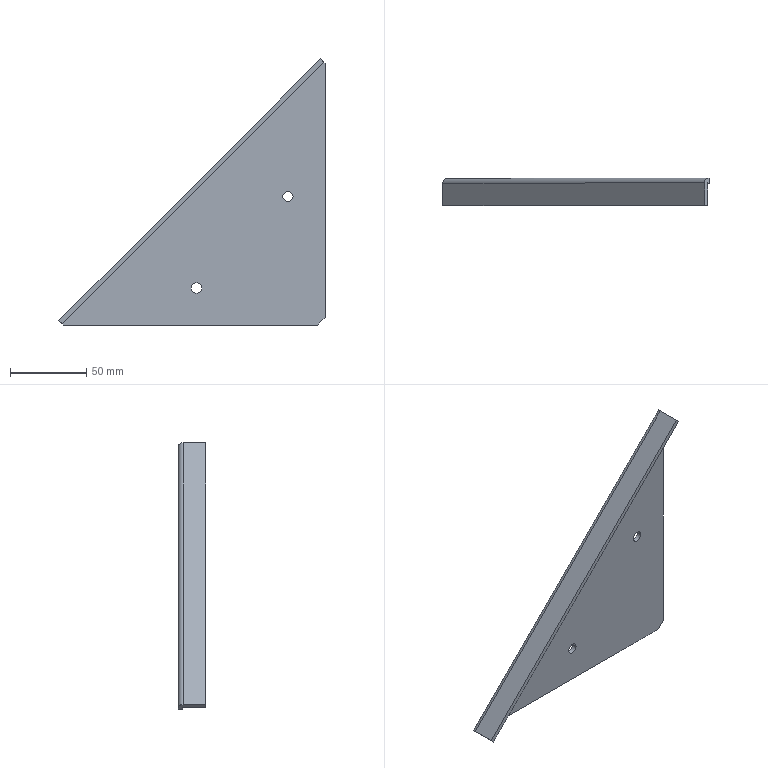Part | STEP file | HESS-408-70-15W-W-18-bottom frame triangular plate | 1 solid | 16 faces | box 175 x 18 x 175 mm | volume 57661 mm3 | plane 10 | cylinder 6 | commonest cylinder face diameters 6.8 x4 0.2 x1 6.2 x1
STEP:
#1=CARTESIAN_POINT('',(0.,0.,0.));
#2=DIRECTION('',(0.,0.,1.));
#3=DIRECTION('',(1.,0.,0.));
#4=AXIS2_PLACEMENT_3D('',#1,#2,#3);
#5=CARTESIAN_POINT('',(-27.826,-3.,84.53));
#6=VERTEX_POINT('',#5);
#7=CARTESIAN_POINT('',(-27.826,0.,84.53));
#8=VERTEX_POINT('',#7);
#9=CARTESIAN_POINT('',(-27.826,0.,84.53));
#10=DIRECTION('',(0.,1.,0.));
#11=VECTOR('',#10,1.);
#12=LINE('',#9,#11);
#13=CARTESIAN_POINT('',(-24.426,0.,84.53));
#14=DIRECTION('',(0.,1.,0.));
#15=DIRECTION('',(-1.,0.,0.));
#16=AXIS2_PLACEMENT_3D('',#13,#14,#15);
#17=CYLINDRICAL_SURFACE('',#16,3.4);
#18=CARTESIAN_POINT('',(6.283,0.));
#19=DIRECTION('',(0.,1.));
#20=VECTOR('',#19,1.);
#21=LINE('',#18,#20);
#22=(GEOMETRIC_REPRESENTATION_CONTEXT(2)PARAMETRIC_REPRESENTATION_CONTEXT()REPRESENTATION_CONTEXT('',''));
#23=DEFINITIONAL_REPRESENTATION('',(#21),#22);
#24=PCURVE('',#17,#23);
#25=CARTESIAN_POINT('',(-24.426,0.,84.53));
#26=DIRECTION('',(0.,1.,0.));
#27=DIRECTION('',(-1.,0.,0.));
#28=AXIS2_PLACEMENT_3D('',#25,#26,#27);
#29=CYLINDRICAL_SURFACE('',#28,3.4);
#30=CARTESIAN_POINT('',(0.,0.));
#31=DIRECTION('',(0.,1.));
#32=VECTOR('',#31,1.);
#33=LINE('',#30,#32);
#34=(GEOMETRIC_REPRESENTATION_CONTEXT(2)PARAMETRIC_REPRESENTATION_CONTEXT()REPRESENTATION_CONTEXT('',''));
#35=DEFINITIONAL_REPRESENTATION('',(#33),#34);
#36=PCURVE('',#29,#35);
#37=SURFACE_CURVE('',#12,(#24,#36),.PCURVE_S1.);
#38=EDGE_CURVE('',#6,#8,#37,.T.);
#39=ORIENTED_EDGE('',*,*,#38,.T.);
#40=CARTESIAN_POINT('',(-21.026,0.,84.53));
#41=VERTEX_POINT('',#40);
#42=CARTESIAN_POINT('',(-24.426,0.,84.53));
#43=DIRECTION('',(0.,-1.,0.));
#44=DIRECTION('',(-1.,0.,0.));
#45=AXIS2_PLACEMENT_3D('',#42,#43,#44);
#46=CIRCLE('',#45,3.4);
#47=CARTESIAN_POINT('',(6.283,0.));
#48=DIRECTION('',(-1.,0.));
#49=VECTOR('',#48,1.);
#50=LINE('',#47,#49);
#51=(GEOMETRIC_REPRESENTATION_CONTEXT(2)PARAMETRIC_REPRESENTATION_CONTEXT()REPRESENTATION_CONTEXT('',''));
#52=DEFINITIONAL_REPRESENTATION('',(#50),#51);
#53=PCURVE('',#17,#52);
#54=CARTESIAN_POINT('',(0.,0.,0.));
#55=DIRECTION('',(0.,1.,0.));
#56=DIRECTION('',(-1.,0.,0.));
#57=AXIS2_PLACEMENT_3D('',#54,#55,#56);
#58=PLANE('',#57);
#59=CARTESIAN_POINT('',(27.826,84.53));
#60=CARTESIAN_POINT('',(27.826,78.642));
#61=CARTESIAN_POINT('',(22.726,81.586));
#62=CARTESIAN_POINT('',(17.626,84.53));
#63=CARTESIAN_POINT('',(22.726,87.475));
#64=CARTESIAN_POINT('',(27.826,90.419));
#65=CARTESIAN_POINT('',(27.826,84.53));
#66=(BOUNDED_CURVE()B_SPLINE_CURVE(2,(#59,#60,#61,#62,#63,#64,#65),.UNSPECIFIED.,.T.,.F.)B_SPLINE_CURVE_WITH_KNOTS((1,2,2,2,2,1),(-2.094,0.,2.094,4.189,6.283,8.378),.UNSPECIFIED.)CURVE()GEOMETRIC_REPRESENTATION_ITEM()RATIONAL_B_SPLINE_CURVE((1.,0.5,1.,0.5,1.,0.5,1.))REPRESENTATION_ITEM(''));
#67=(GEOMETRIC_REPRESENTATION_CONTEXT(2)PARAMETRIC_REPRESENTATION_CONTEXT()REPRESENTATION_CONTEXT('',''));
#68=DEFINITIONAL_REPRESENTATION('',(#66),#67);
#69=PCURVE('',#58,#68);
#70=SURFACE_CURVE('',#46,(#53,#69),.PCURVE_S1.);
#71=EDGE_CURVE('',#8,#41,#70,.T.);
#72=ORIENTED_EDGE('',*,*,#71,.T.);
#73=CARTESIAN_POINT('',(-21.026,-3.,84.53));
#74=VERTEX_POINT('',#73);
#75=CARTESIAN_POINT('',(-21.026,0.,84.53));
#76=DIRECTION('',(0.,1.,0.));
#77=VECTOR('',#76,1.);
#78=LINE('',#75,#77);
#79=CARTESIAN_POINT('',(3.142,0.));
#80=DIRECTION('',(0.,1.));
#81=VECTOR('',#80,1.);
#82=LINE('',#79,#81);
#83=(GEOMETRIC_REPRESENTATION_CONTEXT(2)PARAMETRIC_REPRESENTATION_CONTEXT()REPRESENTATION_CONTEXT('',''));
#84=DEFINITIONAL_REPRESENTATION('',(#82),#83);
#85=PCURVE('',#17,#84);
#86=CARTESIAN_POINT('',(3.142,0.));
#87=DIRECTION('',(0.,1.));
#88=VECTOR('',#87,1.);
#89=LINE('',#86,#88);
#90=(GEOMETRIC_REPRESENTATION_CONTEXT(2)PARAMETRIC_REPRESENTATION_CONTEXT()REPRESENTATION_CONTEXT('',''));
#91=DEFINITIONAL_REPRESENTATION('',(#89),#90);
#92=PCURVE('',#29,#91);
#93=SURFACE_CURVE('',#78,(#85,#92),.PCURVE_S1.);
#94=EDGE_CURVE('',#74,#41,#93,.T.);
#95=ORIENTED_EDGE('',*,*,#94,.F.);
#96=CARTESIAN_POINT('',(-24.426,-3.,84.53));
#97=DIRECTION('',(0.,1.,0.));
#98=DIRECTION('',(-1.,0.,0.));
#99=AXIS2_PLACEMENT_3D('',#96,#97,#98);
#100=CIRCLE('',#99,3.4);
#101=CARTESIAN_POINT('',(0.,-3.));
#102=DIRECTION('',(1.,0.));
#103=VECTOR('',#102,1.);
#104=LINE('',#101,#103);
#105=(GEOMETRIC_REPRESENTATION_CONTEXT(2)PARAMETRIC_REPRESENTATION_CONTEXT()REPRESENTATION_CONTEXT('',''));
#106=DEFINITIONAL_REPRESENTATION('',(#104),#105);
#107=PCURVE('',#17,#106);
#108=CARTESIAN_POINT('',(0.,-3.,0.));
#109=DIRECTION('',(0.,1.,0.));
#110=DIRECTION('',(-1.,0.,0.));
#111=AXIS2_PLACEMENT_3D('',#108,#109,#110);
#112=PLANE('',#111);
#113=CARTESIAN_POINT('',(24.426,84.53));
#114=DIRECTION('',(1.,0.));
#115=AXIS2_PLACEMENT_2D('',#113,#114);
#116=CIRCLE('',#115,3.4);
#117=(GEOMETRIC_REPRESENTATION_CONTEXT(2)PARAMETRIC_REPRESENTATION_CONTEXT()REPRESENTATION_CONTEXT('',''));
#118=DEFINITIONAL_REPRESENTATION('',(#116),#117);
#119=PCURVE('',#112,#118);
#120=SURFACE_CURVE('',#100,(#107,#119),.PCURVE_S1.);
#121=EDGE_CURVE('',#74,#6,#120,.T.);
#122=ORIENTED_EDGE('',*,*,#121,.T.);
#123=EDGE_LOOP('',(#39,#72,#95,#122));
#124=FACE_BOUND('',#123,.F.);
#125=ADVANCED_FACE('',(#124),#17,.F.);
#126=CARTESIAN_POINT('',(-87.93,-3.,24.426));
#127=VERTEX_POINT('',#126);
#128=CARTESIAN_POINT('',(-87.93,0.,24.426));
#129=VERTEX_POINT('',#128);
#130=CARTESIAN_POINT('',(-87.93,0.,24.426));
#131=DIRECTION('',(0.,1.,0.));
#132=VECTOR('',#131,1.);
#133=LINE('',#130,#132);
#134=CARTESIAN_POINT('',(-84.53,0.,24.426));
#135=DIRECTION('',(0.,1.,0.));
#136=DIRECTION('',(-1.,0.,0.));
#137=AXIS2_PLACEMENT_3D('',#134,#135,#136);
#138=CYLINDRICAL_SURFACE('',#137,3.4);
#139=CARTESIAN_POINT('',(6.283,0.));
#140=DIRECTION('',(0.,1.));
#141=VECTOR('',#140,1.);
#142=LINE('',#139,#141);
#143=(GEOMETRIC_REPRESENTATION_CONTEXT(2)PARAMETRIC_REPRESENTATION_CONTEXT()REPRESENTATION_CONTEXT('',''));
#144=DEFINITIONAL_REPRESENTATION('',(#142),#143);
#145=PCURVE('',#138,#144);
#146=CARTESIAN_POINT('',(-84.53,0.,24.426));
#147=DIRECTION('',(0.,1.,0.));
#148=DIRECTION('',(-1.,0.,0.));
#149=AXIS2_PLACEMENT_3D('',#146,#147,#148);
#150=CYLINDRICAL_SURFACE('',#149,3.4);
#151=CARTESIAN_POINT('',(0.,0.));
#152=DIRECTION('',(0.,1.));
#153=VECTOR('',#152,1.);
#154=LINE('',#151,#153);
#155=(GEOMETRIC_REPRESENTATION_CONTEXT(2)PARAMETRIC_REPRESENTATION_CONTEXT()REPRESENTATION_CONTEXT('',''));
#156=DEFINITIONAL_REPRESENTATION('',(#154),#155);
#157=PCURVE('',#150,#156);
#158=SURFACE_CURVE('',#133,(#145,#157),.PCURVE_S1.);
#159=EDGE_CURVE('',#127,#129,#158,.T.);
#160=ORIENTED_EDGE('',*,*,#159,.T.);
#161=CARTESIAN_POINT('',(-81.13,0.,24.426));
#162=VERTEX_POINT('',#161);
#163=CARTESIAN_POINT('',(-84.53,0.,24.426));
#164=DIRECTION('',(0.,-1.,0.));
#165=DIRECTION('',(-1.,0.,0.));
#166=AXIS2_PLACEMENT_3D('',#163,#164,#165);
#167=CIRCLE('',#166,3.4);
#168=CARTESIAN_POINT('',(6.283,0.));
#169=DIRECTION('',(-1.,0.));
#170=VECTOR('',#169,1.);
#171=LINE('',#168,#170);
#172=(GEOMETRIC_REPRESENTATION_CONTEXT(2)PARAMETRIC_REPRESENTATION_CONTEXT()REPRESENTATION_CONTEXT('',''));
#173=DEFINITIONAL_REPRESENTATION('',(#171),#172);
#174=PCURVE('',#138,#173);
#175=CARTESIAN_POINT('',(87.93,24.426));
#176=CARTESIAN_POINT('',(87.93,18.537));
#177=CARTESIAN_POINT('',(82.83,21.482));
#178=CARTESIAN_POINT('',(77.73,24.426));
#179=CARTESIAN_POINT('',(82.83,27.371));
#180=CARTESIAN_POINT('',(87.93,30.315));
#181=CARTESIAN_POINT('',(87.93,24.426));
#182=(BOUNDED_CURVE()B_SPLINE_CURVE(2,(#175,#176,#177,#178,#179,#180,#181),.UNSPECIFIED.,.T.,.F.)B_SPLINE_CURVE_WITH_KNOTS((1,2,2,2,2,1),(-2.094,0.,2.094,4.189,6.283,8.378),.UNSPECIFIED.)CURVE()GEOMETRIC_REPRESENTATION_ITEM()RATIONAL_B_SPLINE_CURVE((1.,0.5,1.,0.5,1.,0.5,1.))REPRESENTATION_ITEM(''));
#183=(GEOMETRIC_REPRESENTATION_CONTEXT(2)PARAMETRIC_REPRESENTATION_CONTEXT()REPRESENTATION_CONTEXT('',''));
#184=DEFINITIONAL_REPRESENTATION('',(#182),#183);
#185=PCURVE('',#58,#184);
#186=SURFACE_CURVE('',#167,(#174,#185),.PCURVE_S1.);
#187=EDGE_CURVE('',#129,#162,#186,.T.);
#188=ORIENTED_EDGE('',*,*,#187,.T.);
#189=CARTESIAN_POINT('',(-81.13,-3.,24.426));
#190=VERTEX_POINT('',#189);
#191=CARTESIAN_POINT('',(-81.13,0.,24.426));
#192=DIRECTION('',(0.,1.,0.));
#193=VECTOR('',#192,1.);
#194=LINE('',#191,#193);
#195=CARTESIAN_POINT('',(3.142,0.));
#196=DIRECTION('',(0.,1.));
#197=VECTOR('',#196,1.);
#198=LINE('',#195,#197);
#199=(GEOMETRIC_REPRESENTATION_CONTEXT(2)PARAMETRIC_REPRESENTATION_CONTEXT()REPRESENTATION_CONTEXT('',''));
#200=DEFINITIONAL_REPRESENTATION('',(#198),#199);
#201=PCURVE('',#138,#200);
#202=CARTESIAN_POINT('',(3.142,0.));
#203=DIRECTION('',(0.,1.));
#204=VECTOR('',#203,1.);
#205=LINE('',#202,#204);
#206=(GEOMETRIC_REPRESENTATION_CONTEXT(2)PARAMETRIC_REPRESENTATION_CONTEXT()REPRESENTATION_CONTEXT('',''));
#207=DEFINITIONAL_REPRESENTATION('',(#205),#206);
#208=PCURVE('',#150,#207);
#209=SURFACE_CURVE('',#194,(#201,#208),.PCURVE_S1.);
#210=EDGE_CURVE('',#190,#162,#209,.T.);
#211=ORIENTED_EDGE('',*,*,#210,.F.);
#212=CARTESIAN_POINT('',(-84.53,-3.,24.426));
#213=DIRECTION('',(0.,1.,0.));
#214=DIRECTION('',(-1.,0.,0.));
#215=AXIS2_PLACEMENT_3D('',#212,#213,#214);
#216=CIRCLE('',#215,3.4);
#217=CARTESIAN_POINT('',(0.,-3.));
#218=DIRECTION('',(1.,0.));
#219=VECTOR('',#218,1.);
#220=LINE('',#217,#219);
#221=(GEOMETRIC_REPRESENTATION_CONTEXT(2)PARAMETRIC_REPRESENTATION_CONTEXT()REPRESENTATION_CONTEXT('',''));
#222=DEFINITIONAL_REPRESENTATION('',(#220),#221);
#223=PCURVE('',#138,#222);
#224=CARTESIAN_POINT('',(84.53,24.426));
#225=DIRECTION('',(1.,0.));
#226=AXIS2_PLACEMENT_2D('',#224,#225);
#227=CIRCLE('',#226,3.4);
#228=(GEOMETRIC_REPRESENTATION_CONTEXT(2)PARAMETRIC_REPRESENTATION_CONTEXT()REPRESENTATION_CONTEXT('',''));
#229=DEFINITIONAL_REPRESENTATION('',(#227),#228);
#230=PCURVE('',#112,#229);
#231=SURFACE_CURVE('',#216,(#223,#230),.PCURVE_S1.);
#232=EDGE_CURVE('',#190,#127,#231,.T.);
#233=ORIENTED_EDGE('',*,*,#232,.T.);
#234=EDGE_LOOP('',(#160,#188,#211,#233));
#235=FACE_BOUND('',#234,.F.);
#236=ADVANCED_FACE('',(#235),#138,.F.);
#237=CARTESIAN_POINT('',(-172.808,0.,0.808));
#238=VERTEX_POINT('',#237);
#239=CARTESIAN_POINT('',(-0.808,0.,172.808));
#240=VERTEX_POINT('',#239);
#241=CARTESIAN_POINT('',(-172.808,0.,0.808));
#242=DIRECTION('',(0.7071,0.,0.7071));
#243=VECTOR('',#242,1.);
#244=LINE('',#241,#243);
#245=CARTESIAN_POINT('',(172.808,0.808));
#246=DIRECTION('',(-0.7071,0.7071));
#247=VECTOR('',#246,1.);
#248=LINE('',#245,#247);
#249=(GEOMETRIC_REPRESENTATION_CONTEXT(2)PARAMETRIC_REPRESENTATION_CONTEXT()REPRESENTATION_CONTEXT('',''));
#250=DEFINITIONAL_REPRESENTATION('',(#248),#249);
#251=PCURVE('',#58,#250);
#252=CARTESIAN_POINT('',(-172.808,-3.1,0.808));
#253=DIRECTION('',(-0.7071,0.,-0.7071));
#254=DIRECTION('',(-0.7071,0.,0.7071));
#255=AXIS2_PLACEMENT_3D('',#252,#253,#254);
#256=CYLINDRICAL_SURFACE('',#255,3.1);
#257=CARTESIAN_POINT('',(1.571,0.));
#258=DIRECTION('',(0.,-1.));
#259=VECTOR('',#258,1.);
#260=LINE('',#257,#259);
#261=(GEOMETRIC_REPRESENTATION_CONTEXT(2)PARAMETRIC_REPRESENTATION_CONTEXT()REPRESENTATION_CONTEXT('',''));
#262=DEFINITIONAL_REPRESENTATION('',(#260),#261);
#263=PCURVE('',#256,#262);
#264=SURFACE_CURVE('',#244,(#251,#263),.PCURVE_S1.);
#265=EDGE_CURVE('',#238,#240,#264,.T.);
#266=ORIENTED_EDGE('',*,*,#265,.T.);
#267=CARTESIAN_POINT('',(0.,0.,172.));
#268=VERTEX_POINT('',#267);
#269=CARTESIAN_POINT('',(-0.808,0.,172.808));
#270=DIRECTION('',(-0.7071,0.,0.7071));
#271=VECTOR('',#270,1.);
#272=LINE('',#269,#271);
#273=CARTESIAN_POINT('',(0.808,172.808));
#274=DIRECTION('',(0.7071,0.7071));
#275=VECTOR('',#274,1.);
#276=LINE('',#273,#275);
#277=(GEOMETRIC_REPRESENTATION_CONTEXT(2)PARAMETRIC_REPRESENTATION_CONTEXT()REPRESENTATION_CONTEXT('',''));
#278=DEFINITIONAL_REPRESENTATION('',(#276),#277);
#279=PCURVE('',#58,#278);
#280=CARTESIAN_POINT('',(-0.808,-3.1,172.808));
#281=DIRECTION('',(0.7071,0.,0.7071));
#282=DIRECTION('',(0.7071,0.,-0.7071));
#283=AXIS2_PLACEMENT_3D('',#280,#281,#282);
#284=PLANE('',#283);
#285=CARTESIAN_POINT('',(0.,3.1));
#286=DIRECTION('',(-1.,0.));
#287=VECTOR('',#286,1.);
#288=LINE('',#285,#287);
#289=(GEOMETRIC_REPRESENTATION_CONTEXT(2)PARAMETRIC_REPRESENTATION_CONTEXT()REPRESENTATION_CONTEXT('',''));
#290=DEFINITIONAL_REPRESENTATION('',(#288),#289);
#291=PCURVE('',#284,#290);
#292=SURFACE_CURVE('',#272,(#279,#291),.PCURVE_S1.);
#293=EDGE_CURVE('',#268,#240,#292,.T.);
#294=ORIENTED_EDGE('',*,*,#293,.F.);
#295=CARTESIAN_POINT('',(0.,0.,5.));
#296=VERTEX_POINT('',#295);
#297=CARTESIAN_POINT('',(0.,0.,0.));
#298=DIRECTION('',(0.,0.,-1.));
#299=VECTOR('',#298,1.);
#300=LINE('',#297,#299);
#301=CARTESIAN_POINT('',(0.,0.));
#302=DIRECTION('',(0.,-1.));
#303=VECTOR('',#302,1.);
#304=LINE('',#301,#303);
#305=(GEOMETRIC_REPRESENTATION_CONTEXT(2)PARAMETRIC_REPRESENTATION_CONTEXT()REPRESENTATION_CONTEXT('',''));
#306=DEFINITIONAL_REPRESENTATION('',(#304),#305);
#307=PCURVE('',#58,#306);
#308=CARTESIAN_POINT('',(0.,-3.,175.));
#309=DIRECTION('',(1.,0.,0.));
#310=DIRECTION('',(0.,1.,0.));
#311=AXIS2_PLACEMENT_3D('',#308,#309,#310);
#312=PLANE('',#311);
#313=CARTESIAN_POINT('',(3.,-175.));
#314=DIRECTION('',(0.,-1.));
#315=VECTOR('',#314,1.);
#316=LINE('',#313,#315);
#317=(GEOMETRIC_REPRESENTATION_CONTEXT(2)PARAMETRIC_REPRESENTATION_CONTEXT()REPRESENTATION_CONTEXT('',''));
#318=DEFINITIONAL_REPRESENTATION('',(#316),#317);
#319=PCURVE('',#312,#318);
#320=SURFACE_CURVE('',#300,(#307,#319),.PCURVE_S1.);
#321=EDGE_CURVE('',#268,#296,#320,.T.);
#322=ORIENTED_EDGE('',*,*,#321,.T.);
#323=CARTESIAN_POINT('',(-5.,0.,0.));
#324=VERTEX_POINT('',#323);
#325=CARTESIAN_POINT('',(0.,0.,5.));
#326=DIRECTION('',(-0.7071,0.,-0.7071));
#327=VECTOR('',#326,1.);
#328=LINE('',#325,#327);
#329=CARTESIAN_POINT('',(0.,5.));
#330=DIRECTION('',(0.7071,-0.7071));
#331=VECTOR('',#330,1.);
#332=LINE('',#329,#331);
#333=(GEOMETRIC_REPRESENTATION_CONTEXT(2)PARAMETRIC_REPRESENTATION_CONTEXT()REPRESENTATION_CONTEXT('',''));
#334=DEFINITIONAL_REPRESENTATION('',(#332),#333);
#335=PCURVE('',#58,#334);
#336=CARTESIAN_POINT('',(0.,-3.,5.));
#337=DIRECTION('',(-0.7071,0.,0.7071));
#338=DIRECTION('',(0.7071,0.,0.7071));
#339=AXIS2_PLACEMENT_3D('',#336,#337,#338);
#340=PLANE('',#339);
#341=CARTESIAN_POINT('',(0.,3.));
#342=DIRECTION('',(-1.,0.));
#343=VECTOR('',#342,1.);
#344=LINE('',#341,#343);
#345=(GEOMETRIC_REPRESENTATION_CONTEXT(2)PARAMETRIC_REPRESENTATION_CONTEXT()REPRESENTATION_CONTEXT('',''));
#346=DEFINITIONAL_REPRESENTATION('',(#344),#345);
#347=PCURVE('',#340,#346);
#348=SURFACE_CURVE('',#328,(#335,#347),.PCURVE_S1.);
#349=EDGE_CURVE('',#296,#324,#348,.T.);
#350=ORIENTED_EDGE('',*,*,#349,.T.);
#351=CARTESIAN_POINT('',(-172.,0.,0.));
#352=VERTEX_POINT('',#351);
#353=CARTESIAN_POINT('',(0.,0.,0.));
#354=DIRECTION('',(-1.,0.,0.));
#355=VECTOR('',#354,1.);
#356=LINE('',#353,#355);
#357=CARTESIAN_POINT('',(0.,0.));
#358=DIRECTION('',(1.,0.));
#359=VECTOR('',#358,1.);
#360=LINE('',#357,#359);
#361=(GEOMETRIC_REPRESENTATION_CONTEXT(2)PARAMETRIC_REPRESENTATION_CONTEXT()REPRESENTATION_CONTEXT('',''));
#362=DEFINITIONAL_REPRESENTATION('',(#360),#361);
#363=PCURVE('',#58,#362);
#364=CARTESIAN_POINT('',(0.,-3.,0.));
#365=DIRECTION('',(0.,0.,-1.));
#366=DIRECTION('',(-1.,0.,0.));
#367=AXIS2_PLACEMENT_3D('',#364,#365,#366);
#368=PLANE('',#367);
#369=CARTESIAN_POINT('',(0.,3.));
#370=DIRECTION('',(1.,0.));
#371=VECTOR('',#370,1.);
#372=LINE('',#369,#371);
#373=(GEOMETRIC_REPRESENTATION_CONTEXT(2)PARAMETRIC_REPRESENTATION_CONTEXT()REPRESENTATION_CONTEXT('',''));
#374=DEFINITIONAL_REPRESENTATION('',(#372),#373);
#375=PCURVE('',#368,#374);
#376=SURFACE_CURVE('',#356,(#363,#375),.PCURVE_S1.);
#377=EDGE_CURVE('',#324,#352,#376,.T.);
#378=ORIENTED_EDGE('',*,*,#377,.T.);
#379=CARTESIAN_POINT('',(-172.596,0.,0.5958));
#380=DIRECTION('',(0.7071,0.,-0.7071));
#381=VECTOR('',#380,1.);
#382=LINE('',#379,#381);
#383=CARTESIAN_POINT('',(172.596,0.5958));
#384=DIRECTION('',(-0.7071,-0.7071));
#385=VECTOR('',#384,1.);
#386=LINE('',#383,#385);
#387=(GEOMETRIC_REPRESENTATION_CONTEXT(2)PARAMETRIC_REPRESENTATION_CONTEXT()REPRESENTATION_CONTEXT('',''));
#388=DEFINITIONAL_REPRESENTATION('',(#386),#387);
#389=PCURVE('',#58,#388);
#390=CARTESIAN_POINT('',(-172.808,-3.1,0.808));
#391=DIRECTION('',(0.7071,0.,0.7071));
#392=DIRECTION('',(0.7071,0.,-0.7071));
#393=AXIS2_PLACEMENT_3D('',#390,#391,#392);
#394=PLANE('',#393);
#395=CARTESIAN_POINT('',(0.3,3.1));
#396=DIRECTION('',(1.,0.));
#397=VECTOR('',#396,1.);
#398=LINE('',#395,#397);
#399=(GEOMETRIC_REPRESENTATION_CONTEXT(2)PARAMETRIC_REPRESENTATION_CONTEXT()REPRESENTATION_CONTEXT('',''));
#400=DEFINITIONAL_REPRESENTATION('',(#398),#399);
#401=PCURVE('',#394,#400);
#402=SURFACE_CURVE('',#382,(#389,#401),.PCURVE_S1.);
#403=EDGE_CURVE('',#238,#352,#402,.T.);
#404=ORIENTED_EDGE('',*,*,#403,.F.);
#405=EDGE_LOOP('',(#266,#294,#322,#350,#378,#404));
#406=FACE_BOUND('',#405,.T.);
#407=ORIENTED_EDGE('',*,*,#71,.T.);
#408=CARTESIAN_POINT('',(-24.426,0.,84.53));
#409=DIRECTION('',(0.,-1.,0.));
#410=DIRECTION('',(-1.,0.,0.));
#411=AXIS2_PLACEMENT_3D('',#408,#409,#410);
#412=CIRCLE('',#411,3.4);
#413=CARTESIAN_POINT('',(27.826,84.53));
#414=CARTESIAN_POINT('',(27.826,78.642));
#415=CARTESIAN_POINT('',(22.726,81.586));
#416=CARTESIAN_POINT('',(17.626,84.53));
#417=CARTESIAN_POINT('',(22.726,87.475));
#418=CARTESIAN_POINT('',(27.826,90.419));
#419=CARTESIAN_POINT('',(27.826,84.53));
#420=(BOUNDED_CURVE()B_SPLINE_CURVE(2,(#413,#414,#415,#416,#417,#418,#419),.UNSPECIFIED.,.T.,.F.)B_SPLINE_CURVE_WITH_KNOTS((1,2,2,2,2,1),(-2.094,0.,2.094,4.189,6.283,8.378),.UNSPECIFIED.)CURVE()GEOMETRIC_REPRESENTATION_ITEM()RATIONAL_B_SPLINE_CURVE((1.,0.5,1.,0.5,1.,0.5,1.))REPRESENTATION_ITEM(''));
#421=(GEOMETRIC_REPRESENTATION_CONTEXT(2)PARAMETRIC_REPRESENTATION_CONTEXT()REPRESENTATION_CONTEXT('',''));
#422=DEFINITIONAL_REPRESENTATION('',(#420),#421);
#423=PCURVE('',#58,#422);
#424=CARTESIAN_POINT('',(6.283,0.));
#425=DIRECTION('',(-1.,0.));
#426=VECTOR('',#425,1.);
#427=LINE('',#424,#426);
#428=(GEOMETRIC_REPRESENTATION_CONTEXT(2)PARAMETRIC_REPRESENTATION_CONTEXT()REPRESENTATION_CONTEXT('',''));
#429=DEFINITIONAL_REPRESENTATION('',(#427),#428);
#430=PCURVE('',#29,#429);
#431=SURFACE_CURVE('',#412,(#423,#430),.PCURVE_S1.);
#432=EDGE_CURVE('',#41,#8,#431,.T.);
#433=ORIENTED_EDGE('',*,*,#432,.T.);
#434=EDGE_LOOP('',(#407,#433));
#435=FACE_BOUND('',#434,.T.);
#436=ORIENTED_EDGE('',*,*,#187,.T.);
#437=CARTESIAN_POINT('',(-84.53,0.,24.426));
#438=DIRECTION('',(0.,-1.,0.));
#439=DIRECTION('',(-1.,0.,0.));
#440=AXIS2_PLACEMENT_3D('',#437,#438,#439);
#441=CIRCLE('',#440,3.4);
#442=CARTESIAN_POINT('',(87.93,24.426));
#443=CARTESIAN_POINT('',(87.93,18.537));
#444=CARTESIAN_POINT('',(82.83,21.482));
#445=CARTESIAN_POINT('',(77.73,24.426));
#446=CARTESIAN_POINT('',(82.83,27.371));
#447=CARTESIAN_POINT('',(87.93,30.315));
#448=CARTESIAN_POINT('',(87.93,24.426));
#449=(BOUNDED_CURVE()B_SPLINE_CURVE(2,(#442,#443,#444,#445,#446,#447,#448),.UNSPECIFIED.,.T.,.F.)B_SPLINE_CURVE_WITH_KNOTS((1,2,2,2,2,1),(-2.094,0.,2.094,4.189,6.283,8.378),.UNSPECIFIED.)CURVE()GEOMETRIC_REPRESENTATION_ITEM()RATIONAL_B_SPLINE_CURVE((1.,0.5,1.,0.5,1.,0.5,1.))REPRESENTATION_ITEM(''));
#450=(GEOMETRIC_REPRESENTATION_CONTEXT(2)PARAMETRIC_REPRESENTATION_CONTEXT()REPRESENTATION_CONTEXT('',''));
#451=DEFINITIONAL_REPRESENTATION('',(#449),#450);
#452=PCURVE('',#58,#451);
#453=CARTESIAN_POINT('',(6.283,0.));
#454=DIRECTION('',(-1.,0.));
#455=VECTOR('',#454,1.);
#456=LINE('',#453,#455);
#457=(GEOMETRIC_REPRESENTATION_CONTEXT(2)PARAMETRIC_REPRESENTATION_CONTEXT()REPRESENTATION_CONTEXT('',''));
#458=DEFINITIONAL_REPRESENTATION('',(#456),#457);
#459=PCURVE('',#150,#458);
#460=SURFACE_CURVE('',#441,(#452,#459),.PCURVE_S1.);
#461=EDGE_CURVE('',#162,#129,#460,.T.);
#462=ORIENTED_EDGE('',*,*,#461,.T.);
#463=EDGE_LOOP('',(#436,#462));
#464=FACE_BOUND('',#463,.T.);
#465=ADVANCED_FACE('',(#406,#435,#464),#58,.T.);
#466=CARTESIAN_POINT('',(-175.,-3.1,3.));
#467=VERTEX_POINT('',#466);
#468=CARTESIAN_POINT('',(-3.,-3.1,175.));
#469=VERTEX_POINT('',#468);
#470=CARTESIAN_POINT('',(-175.,-3.1,3.));
#471=DIRECTION('',(0.7071,0.,0.7071));
#472=VECTOR('',#471,1.);
#473=LINE('',#470,#472);
#474=CARTESIAN_POINT('',(0.,0.));
#475=CARTESIAN_POINT('',(0.,-3.686));
#476=CARTESIAN_POINT('',(0.,-11.057));
#477=CARTESIAN_POINT('',(0.,-22.113));
#478=CARTESIAN_POINT('',(0.,-33.17));
#479=CARTESIAN_POINT('',(0.,-44.226));
#480=CARTESIAN_POINT('',(0.,-55.283));
#481=CARTESIAN_POINT('',(0.,-66.339));
#482=CARTESIAN_POINT('',(0.,-77.396));
#483=CARTESIAN_POINT('',(0.,-88.453));
#484=CARTESIAN_POINT('',(0.,-99.509));
#485=CARTESIAN_POINT('',(0.,-110.566));
#486=CARTESIAN_POINT('',(0.,-121.622));
#487=CARTESIAN_POINT('',(0.,-132.679));
#488=CARTESIAN_POINT('',(0.,-143.736));
#489=CARTESIAN_POINT('',(0.,-154.792));
#490=CARTESIAN_POINT('',(0.,-165.849));
#491=CARTESIAN_POINT('',(0.,-176.905));
#492=CARTESIAN_POINT('',(0.,-187.962));
#493=CARTESIAN_POINT('',(0.,-199.018));
#494=CARTESIAN_POINT('',(0.,-210.075));
#495=CARTESIAN_POINT('',(0.,-221.132));
#496=CARTESIAN_POINT('',(0.,-232.188));
#497=CARTESIAN_POINT('',(0.,-239.559));
#498=CARTESIAN_POINT('',(0.,-243.245));
#499=B_SPLINE_CURVE_WITH_KNOTS('',3,(#474,#475,#476,#477,#478,#479,#480,#481,#482,#483,#484,#485,#486,#487,#488,#489,#490,#491,#492,#493,#494,#495,#496,#497,#498),.UNSPECIFIED.,.F.,.F.,(4,1,1,1,1,1,1,1,1,1,1,1,1,1,1,1,1,1,1,1,1,1,4),(0.,11.057,22.113,33.17,44.226,55.283,66.339,77.396,88.453,99.509,110.566,121.622,132.679,143.736,154.792,165.849,176.905,187.962,199.018,210.075,221.132,232.188,243.245),.QUASI_UNIFORM_KNOTS.);
#500=(GEOMETRIC_REPRESENTATION_CONTEXT(2)PARAMETRIC_REPRESENTATION_CONTEXT()REPRESENTATION_CONTEXT('',''));
#501=DEFINITIONAL_REPRESENTATION('',(#499),#500);
#502=PCURVE('',#256,#501);
#503=CARTESIAN_POINT('',(-89.,0.,89.));
#504=DIRECTION('',(-0.7071,0.,0.7071));
#505=DIRECTION('',(0.7071,0.,0.7071));
#506=AXIS2_PLACEMENT_3D('',#503,#504,#505);
#507=PLANE('',#506);
#508=CARTESIAN_POINT('',(-121.622,-3.1));
#509=DIRECTION('',(1.,0.));
#510=VECTOR('',#509,1.);
#511=LINE('',#508,#510);
#512=(GEOMETRIC_REPRESENTATION_CONTEXT(2)PARAMETRIC_REPRESENTATION_CONTEXT()REPRESENTATION_CONTEXT('',''));
#513=DEFINITIONAL_REPRESENTATION('',(#511),#512);
#514=PCURVE('',#507,#513);
#515=SURFACE_CURVE('',#473,(#502,#514),.PCURVE_S1.);
#516=EDGE_CURVE('',#467,#469,#515,.T.);
#517=ORIENTED_EDGE('',*,*,#516,.T.);
#518=CARTESIAN_POINT('',(-0.808,-3.1,172.808));
#519=DIRECTION('',(-0.7071,0.,-0.7071));
#520=DIRECTION('',(-0.7071,0.,0.7071));
#521=AXIS2_PLACEMENT_3D('',#518,#519,#520);
#522=CIRCLE('',#521,3.1);
#523=CARTESIAN_POINT('',(0.,-243.245));
#524=DIRECTION('',(1.,0.));
#525=VECTOR('',#524,1.);
#526=LINE('',#523,#525);
#527=(GEOMETRIC_REPRESENTATION_CONTEXT(2)PARAMETRIC_REPRESENTATION_CONTEXT()REPRESENTATION_CONTEXT('',''));
#528=DEFINITIONAL_REPRESENTATION('',(#526),#527);
#529=PCURVE('',#256,#528);
#530=CARTESIAN_POINT('',(-3.1,0.));
#531=CARTESIAN_POINT('',(-3.1,5.369));
#532=CARTESIAN_POINT('',(1.55,2.685));
#533=CARTESIAN_POINT('',(6.2,0.));
#534=CARTESIAN_POINT('',(1.55,-2.685));
#535=CARTESIAN_POINT('',(-3.1,-5.369));
#536=CARTESIAN_POINT('',(-3.1,0.));
#537=(BOUNDED_CURVE()B_SPLINE_CURVE(2,(#530,#531,#532,#533,#534,#535,#536),.UNSPECIFIED.,.T.,.F.)B_SPLINE_CURVE_WITH_KNOTS((1,2,2,2,2,1),(-2.094,0.,2.094,4.189,6.283,8.378),.UNSPECIFIED.)CURVE()GEOMETRIC_REPRESENTATION_ITEM()RATIONAL_B_SPLINE_CURVE((1.,0.5,1.,0.5,1.,0.5,1.))REPRESENTATION_ITEM(''));
#538=(GEOMETRIC_REPRESENTATION_CONTEXT(2)PARAMETRIC_REPRESENTATION_CONTEXT()REPRESENTATION_CONTEXT('',''));
#539=DEFINITIONAL_REPRESENTATION('',(#537),#538);
#540=PCURVE('',#284,#539);
#541=SURFACE_CURVE('',#522,(#529,#540),.PCURVE_S1.);
#542=EDGE_CURVE('',#469,#240,#541,.T.);
#543=ORIENTED_EDGE('',*,*,#542,.T.);
#544=ORIENTED_EDGE('',*,*,#265,.F.);
#545=CARTESIAN_POINT('',(-172.808,-3.1,0.808));
#546=DIRECTION('',(0.7071,0.,0.7071));
#547=DIRECTION('',(-0.7071,0.,0.7071));
#548=AXIS2_PLACEMENT_3D('',#545,#546,#547);
#549=CIRCLE('',#548,3.1);
#550=CARTESIAN_POINT('',(6.283,0.));
#551=DIRECTION('',(-1.,0.));
#552=VECTOR('',#551,1.);
#553=LINE('',#550,#552);
#554=(GEOMETRIC_REPRESENTATION_CONTEXT(2)PARAMETRIC_REPRESENTATION_CONTEXT()REPRESENTATION_CONTEXT('',''));
#555=DEFINITIONAL_REPRESENTATION('',(#553),#554);
#556=PCURVE('',#256,#555);
#557=CARTESIAN_POINT('',(0.,0.));
#558=DIRECTION('',(-1.,0.));
#559=AXIS2_PLACEMENT_2D('',#557,#558);
#560=CIRCLE('',#559,3.1);
#561=(GEOMETRIC_REPRESENTATION_CONTEXT(2)PARAMETRIC_REPRESENTATION_CONTEXT()REPRESENTATION_CONTEXT('',''));
#562=DEFINITIONAL_REPRESENTATION('',(#560),#561);
#563=PCURVE('',#394,#562);
#564=SURFACE_CURVE('',#549,(#556,#563),.PCURVE_S1.);
#565=EDGE_CURVE('',#238,#467,#564,.T.);
#566=ORIENTED_EDGE('',*,*,#565,.T.);
#567=EDGE_LOOP('',(#517,#543,#544,#566));
#568=FACE_BOUND('',#567,.T.);
#569=ADVANCED_FACE('',(#568),#256,.T.);
#570=CARTESIAN_POINT('',(-5.,-3.,0.));
#571=VERTEX_POINT('',#570);
#572=CARTESIAN_POINT('',(-172.,-3.,0.));
#573=VERTEX_POINT('',#572);
#574=CARTESIAN_POINT('',(0.,-3.,0.));
#575=DIRECTION('',(-1.,0.,0.));
#576=VECTOR('',#575,1.);
#577=LINE('',#574,#576);
#578=CARTESIAN_POINT('',(0.,0.));
#579=DIRECTION('',(1.,0.));
#580=VECTOR('',#579,1.);
#581=LINE('',#578,#580);
#582=(GEOMETRIC_REPRESENTATION_CONTEXT(2)PARAMETRIC_REPRESENTATION_CONTEXT()REPRESENTATION_CONTEXT('',''));
#583=DEFINITIONAL_REPRESENTATION('',(#581),#582);
#584=PCURVE('',#368,#583);
#585=CARTESIAN_POINT('',(0.,0.));
#586=DIRECTION('',(1.,0.));
#587=VECTOR('',#586,1.);
#588=LINE('',#585,#587);
#589=(GEOMETRIC_REPRESENTATION_CONTEXT(2)PARAMETRIC_REPRESENTATION_CONTEXT()REPRESENTATION_CONTEXT('',''));
#590=DEFINITIONAL_REPRESENTATION('',(#588),#589);
#591=PCURVE('',#112,#590);
#592=SURFACE_CURVE('',#577,(#584,#591),.PCURVE_S1.);
#593=EDGE_CURVE('',#571,#573,#592,.T.);
#594=ORIENTED_EDGE('',*,*,#593,.T.);
#595=CARTESIAN_POINT('',(-172.,-3.,0.));
#596=DIRECTION('',(0.,1.,0.));
#597=VECTOR('',#596,1.);
#598=LINE('',#595,#597);
#599=CARTESIAN_POINT('',(172.,0.));
#600=DIRECTION('',(0.,1.));
#601=VECTOR('',#600,1.);
#602=LINE('',#599,#601);
#603=(GEOMETRIC_REPRESENTATION_CONTEXT(2)PARAMETRIC_REPRESENTATION_CONTEXT()REPRESENTATION_CONTEXT('',''));
#604=DEFINITIONAL_REPRESENTATION('',(#602),#603);
#605=PCURVE('',#368,#604);
#606=CARTESIAN_POINT('',(1.143,0.1));
#607=DIRECTION('',(0.,1.));
#608=VECTOR('',#607,1.);
#609=LINE('',#606,#608);
#610=(GEOMETRIC_REPRESENTATION_CONTEXT(2)PARAMETRIC_REPRESENTATION_CONTEXT()REPRESENTATION_CONTEXT('',''));
#611=DEFINITIONAL_REPRESENTATION('',(#609),#610);
#612=PCURVE('',#394,#611);
#613=SURFACE_CURVE('',#598,(#605,#612),.PCURVE_S1.);
#614=EDGE_CURVE('',#573,#352,#613,.T.);
#615=ORIENTED_EDGE('',*,*,#614,.T.);
#616=ORIENTED_EDGE('',*,*,#377,.F.);
#617=CARTESIAN_POINT('',(-5.,-3.,0.));
#618=DIRECTION('',(0.,-1.,0.));
#619=VECTOR('',#618,1.);
#620=LINE('',#617,#619);
#621=CARTESIAN_POINT('',(5.,0.));
#622=DIRECTION('',(0.,-1.));
#623=VECTOR('',#622,1.);
#624=LINE('',#621,#623);
#625=(GEOMETRIC_REPRESENTATION_CONTEXT(2)PARAMETRIC_REPRESENTATION_CONTEXT()REPRESENTATION_CONTEXT('',''));
#626=DEFINITIONAL_REPRESENTATION('',(#624),#625);
#627=PCURVE('',#368,#626);
#628=CARTESIAN_POINT('',(-7.071,0.));
#629=DIRECTION('',(0.,-1.));
#630=VECTOR('',#629,1.);
#631=LINE('',#628,#630);
#632=(GEOMETRIC_REPRESENTATION_CONTEXT(2)PARAMETRIC_REPRESENTATION_CONTEXT()REPRESENTATION_CONTEXT('',''));
#633=DEFINITIONAL_REPRESENTATION('',(#631),#632);
#634=PCURVE('',#340,#633);
#635=SURFACE_CURVE('',#620,(#627,#634),.PCURVE_S1.);
#636=EDGE_CURVE('',#324,#571,#635,.T.);
#637=ORIENTED_EDGE('',*,*,#636,.T.);
#638=EDGE_LOOP('',(#594,#615,#616,#637));
#639=FACE_BOUND('',#638,.T.);
#640=ADVANCED_FACE('',(#639),#368,.T.);
#641=ORIENTED_EDGE('',*,*,#636,.F.);
#642=ORIENTED_EDGE('',*,*,#349,.F.);
#643=CARTESIAN_POINT('',(0.,-3.,5.));
#644=VERTEX_POINT('',#643);
#645=CARTESIAN_POINT('',(0.,-3.,5.));
#646=DIRECTION('',(0.,1.,0.));
#647=VECTOR('',#646,1.);
#648=LINE('',#645,#647);
#649=CARTESIAN_POINT('',(0.,0.));
#650=DIRECTION('',(0.,1.));
#651=VECTOR('',#650,1.);
#652=LINE('',#649,#651);
#653=(GEOMETRIC_REPRESENTATION_CONTEXT(2)PARAMETRIC_REPRESENTATION_CONTEXT()REPRESENTATION_CONTEXT('',''));
#654=DEFINITIONAL_REPRESENTATION('',(#652),#653);
#655=PCURVE('',#340,#654);
#656=CARTESIAN_POINT('',(0.,-170.));
#657=DIRECTION('',(1.,0.));
#658=VECTOR('',#657,1.);
#659=LINE('',#656,#658);
#660=(GEOMETRIC_REPRESENTATION_CONTEXT(2)PARAMETRIC_REPRESENTATION_CONTEXT()REPRESENTATION_CONTEXT('',''));
#661=DEFINITIONAL_REPRESENTATION('',(#659),#660);
#662=PCURVE('',#312,#661);
#663=SURFACE_CURVE('',#648,(#655,#662),.PCURVE_S1.);
#664=EDGE_CURVE('',#644,#296,#663,.T.);
#665=ORIENTED_EDGE('',*,*,#664,.F.);
#666=CARTESIAN_POINT('',(0.,-3.,5.));
#667=DIRECTION('',(0.7071,0.,0.7071));
#668=VECTOR('',#667,1.);
#669=LINE('',#666,#668);
#670=CARTESIAN_POINT('',(0.,0.));
#671=DIRECTION('',(1.,0.));
#672=VECTOR('',#671,1.);
#673=LINE('',#670,#672);
#674=(GEOMETRIC_REPRESENTATION_CONTEXT(2)PARAMETRIC_REPRESENTATION_CONTEXT()REPRESENTATION_CONTEXT('',''));
#675=DEFINITIONAL_REPRESENTATION('',(#673),#674);
#676=PCURVE('',#340,#675);
#677=CARTESIAN_POINT('',(0.,5.));
#678=DIRECTION('',(-0.7071,0.7071));
#679=VECTOR('',#678,1.);
#680=LINE('',#677,#679);
#681=(GEOMETRIC_REPRESENTATION_CONTEXT(2)PARAMETRIC_REPRESENTATION_CONTEXT()REPRESENTATION_CONTEXT('',''));
#682=DEFINITIONAL_REPRESENTATION('',(#680),#681);
#683=PCURVE('',#112,#682);
#684=SURFACE_CURVE('',#669,(#676,#683),.PCURVE_S1.);
#685=EDGE_CURVE('',#571,#644,#684,.T.);
#686=ORIENTED_EDGE('',*,*,#685,.F.);
#687=EDGE_LOOP('',(#641,#642,#665,#686));
#688=FACE_BOUND('',#687,.T.);
#689=ADVANCED_FACE('',(#688),#340,.F.);
#690=ORIENTED_EDGE('',*,*,#321,.F.);
#691=CARTESIAN_POINT('',(0.,-3.,172.));
#692=VERTEX_POINT('',#691);
#693=CARTESIAN_POINT('',(0.,-3.,172.));
#694=DIRECTION('',(0.,-1.,0.));
#695=VECTOR('',#694,1.);
#696=LINE('',#693,#695);
#697=CARTESIAN_POINT('',(0.,-3.));
#698=DIRECTION('',(-1.,0.));
#699=VECTOR('',#698,1.);
#700=LINE('',#697,#699);
#701=(GEOMETRIC_REPRESENTATION_CONTEXT(2)PARAMETRIC_REPRESENTATION_CONTEXT()REPRESENTATION_CONTEXT('',''));
#702=DEFINITIONAL_REPRESENTATION('',(#700),#701);
#703=PCURVE('',#312,#702);
#704=CARTESIAN_POINT('',(1.143,0.1));
#705=DIRECTION('',(0.,-1.));
#706=VECTOR('',#705,1.);
#707=LINE('',#704,#706);
#708=(GEOMETRIC_REPRESENTATION_CONTEXT(2)PARAMETRIC_REPRESENTATION_CONTEXT()REPRESENTATION_CONTEXT('',''));
#709=DEFINITIONAL_REPRESENTATION('',(#707),#708);
#710=PCURVE('',#284,#709);
#711=SURFACE_CURVE('',#696,(#703,#710),.PCURVE_S1.);
#712=EDGE_CURVE('',#268,#692,#711,.T.);
#713=ORIENTED_EDGE('',*,*,#712,.T.);
#714=CARTESIAN_POINT('',(0.,-3.,175.));
#715=DIRECTION('',(0.,0.,-1.));
#716=VECTOR('',#715,1.);
#717=LINE('',#714,#716);
#718=CARTESIAN_POINT('',(0.,0.));
#719=DIRECTION('',(0.,-1.));
#720=VECTOR('',#719,1.);
#721=LINE('',#718,#720);
#722=(GEOMETRIC_REPRESENTATION_CONTEXT(2)PARAMETRIC_REPRESENTATION_CONTEXT()REPRESENTATION_CONTEXT('',''));
#723=DEFINITIONAL_REPRESENTATION('',(#721),#722);
#724=PCURVE('',#312,#723);
#725=CARTESIAN_POINT('',(0.,175.));
#726=DIRECTION('',(0.,-1.));
#727=VECTOR('',#726,1.);
#728=LINE('',#725,#727);
#729=(GEOMETRIC_REPRESENTATION_CONTEXT(2)PARAMETRIC_REPRESENTATION_CONTEXT()REPRESENTATION_CONTEXT('',''));
#730=DEFINITIONAL_REPRESENTATION('',(#728),#729);
#731=PCURVE('',#112,#730);
#732=SURFACE_CURVE('',#717,(#724,#731),.PCURVE_S1.);
#733=EDGE_CURVE('',#692,#644,#732,.T.);
#734=ORIENTED_EDGE('',*,*,#733,.T.);
#735=ORIENTED_EDGE('',*,*,#664,.T.);
#736=EDGE_LOOP('',(#690,#713,#734,#735));
#737=FACE_BOUND('',#736,.T.);
#738=ADVANCED_FACE('',(#737),#312,.T.);
#739=ORIENTED_EDGE('',*,*,#432,.T.);
#740=ORIENTED_EDGE('',*,*,#38,.F.);
#741=CARTESIAN_POINT('',(-24.426,-3.,84.53));
#742=DIRECTION('',(0.,1.,0.));
#743=DIRECTION('',(-1.,0.,0.));
#744=AXIS2_PLACEMENT_3D('',#741,#742,#743);
#745=CIRCLE('',#744,3.4);
#746=CARTESIAN_POINT('',(0.,-3.));
#747=DIRECTION('',(1.,0.));
#748=VECTOR('',#747,1.);
#749=LINE('',#746,#748);
#750=(GEOMETRIC_REPRESENTATION_CONTEXT(2)PARAMETRIC_REPRESENTATION_CONTEXT()REPRESENTATION_CONTEXT('',''));
#751=DEFINITIONAL_REPRESENTATION('',(#749),#750);
#752=PCURVE('',#29,#751);
#753=CARTESIAN_POINT('',(24.426,84.53));
#754=DIRECTION('',(1.,0.));
#755=AXIS2_PLACEMENT_2D('',#753,#754);
#756=CIRCLE('',#755,3.4);
#757=(GEOMETRIC_REPRESENTATION_CONTEXT(2)PARAMETRIC_REPRESENTATION_CONTEXT()REPRESENTATION_CONTEXT('',''));
#758=DEFINITIONAL_REPRESENTATION('',(#756),#757);
#759=PCURVE('',#112,#758);
#760=SURFACE_CURVE('',#745,(#752,#759),.PCURVE_S1.);
#761=EDGE_CURVE('',#6,#74,#760,.T.);
#762=ORIENTED_EDGE('',*,*,#761,.T.);
#763=ORIENTED_EDGE('',*,*,#94,.T.);
#764=EDGE_LOOP('',(#739,#740,#762,#763));
#765=FACE_BOUND('',#764,.F.);
#766=ADVANCED_FACE('',(#765),#29,.F.);
#767=ORIENTED_EDGE('',*,*,#461,.T.);
#768=ORIENTED_EDGE('',*,*,#159,.F.);
#769=CARTESIAN_POINT('',(-84.53,-3.,24.426));
#770=DIRECTION('',(0.,1.,0.));
#771=DIRECTION('',(-1.,0.,0.));
#772=AXIS2_PLACEMENT_3D('',#769,#770,#771);
#773=CIRCLE('',#772,3.4);
#774=CARTESIAN_POINT('',(0.,-3.));
#775=DIRECTION('',(1.,0.));
#776=VECTOR('',#775,1.);
#777=LINE('',#774,#776);
#778=(GEOMETRIC_REPRESENTATION_CONTEXT(2)PARAMETRIC_REPRESENTATION_CONTEXT()REPRESENTATION_CONTEXT('',''));
#779=DEFINITIONAL_REPRESENTATION('',(#777),#778);
#780=PCURVE('',#150,#779);
#781=CARTESIAN_POINT('',(84.53,24.426));
#782=DIRECTION('',(1.,0.));
#783=AXIS2_PLACEMENT_2D('',#781,#782);
#784=CIRCLE('',#783,3.4);
#785=(GEOMETRIC_REPRESENTATION_CONTEXT(2)PARAMETRIC_REPRESENTATION_CONTEXT()REPRESENTATION_CONTEXT('',''));
#786=DEFINITIONAL_REPRESENTATION('',(#784),#785);
#787=PCURVE('',#112,#786);
#788=SURFACE_CURVE('',#773,(#780,#787),.PCURVE_S1.);
#789=EDGE_CURVE('',#127,#190,#788,.T.);
#790=ORIENTED_EDGE('',*,*,#789,.T.);
#791=ORIENTED_EDGE('',*,*,#210,.T.);
#792=EDGE_LOOP('',(#767,#768,#790,#791));
#793=FACE_BOUND('',#792,.F.);
#794=ADVANCED_FACE('',(#793),#150,.F.);
#795=CARTESIAN_POINT('',(-0.8787,-3.1,172.879));
#796=VERTEX_POINT('',#795);
#797=CARTESIAN_POINT('',(-0.808,-3.,172.808));
#798=VERTEX_POINT('',#797);
#799=CARTESIAN_POINT('',(-0.808,-3.1,172.808));
#800=DIRECTION('',(-0.7071,0.,-0.7071));
#801=DIRECTION('',(-0.7071,0.,0.7071));
#802=AXIS2_PLACEMENT_3D('',#799,#800,#801);
#803=CIRCLE('',#802,0.1);
#804=CARTESIAN_POINT('',(-0.1,0.));
#805=CARTESIAN_POINT('',(-0.1,0.1732));
#806=CARTESIAN_POINT('',(0.05,0.0866));
#807=CARTESIAN_POINT('',(0.2,0.));
#808=CARTESIAN_POINT('',(0.05,-0.0866));
#809=CARTESIAN_POINT('',(-0.1,-0.1732));
#810=CARTESIAN_POINT('',(-0.1,0.));
#811=(BOUNDED_CURVE()B_SPLINE_CURVE(2,(#804,#805,#806,#807,#808,#809,#810),.UNSPECIFIED.,.T.,.F.)B_SPLINE_CURVE_WITH_KNOTS((1,2,2,2,2,1),(-2.094,0.,2.094,4.189,6.283,8.378),.UNSPECIFIED.)CURVE()GEOMETRIC_REPRESENTATION_ITEM()RATIONAL_B_SPLINE_CURVE((1.,0.5,1.,0.5,1.,0.5,1.))REPRESENTATION_ITEM(''));
#812=(GEOMETRIC_REPRESENTATION_CONTEXT(2)PARAMETRIC_REPRESENTATION_CONTEXT()REPRESENTATION_CONTEXT('',''));
#813=DEFINITIONAL_REPRESENTATION('',(#811),#812);
#814=PCURVE('',#284,#813);
#815=CARTESIAN_POINT('',(-172.808,-3.1,0.808));
#816=DIRECTION('',(-0.7071,0.,-0.7071));
#817=DIRECTION('',(-0.7071,0.,0.7071));
#818=AXIS2_PLACEMENT_3D('',#815,#816,#817);
#819=CYLINDRICAL_SURFACE('',#818,0.1);
#820=CARTESIAN_POINT('',(0.,-243.245));
#821=DIRECTION('',(1.,0.));
#822=VECTOR('',#821,1.);
#823=LINE('',#820,#822);
#824=(GEOMETRIC_REPRESENTATION_CONTEXT(2)PARAMETRIC_REPRESENTATION_CONTEXT()REPRESENTATION_CONTEXT('',''));
#825=DEFINITIONAL_REPRESENTATION('',(#823),#824);
#826=PCURVE('',#819,#825);
#827=SURFACE_CURVE('',#803,(#814,#826),.PCURVE_S1.);
#828=EDGE_CURVE('',#796,#798,#827,.T.);
#829=ORIENTED_EDGE('',*,*,#828,.T.);
#830=CARTESIAN_POINT('',(-0.808,-3.,172.808));
#831=DIRECTION('',(0.7071,0.,-0.7071));
#832=VECTOR('',#831,1.);
#833=LINE('',#830,#832);
#834=CARTESIAN_POINT('',(0.,0.1));
#835=DIRECTION('',(1.,0.));
#836=VECTOR('',#835,1.);
#837=LINE('',#834,#836);
#838=(GEOMETRIC_REPRESENTATION_CONTEXT(2)PARAMETRIC_REPRESENTATION_CONTEXT()REPRESENTATION_CONTEXT('',''));
#839=DEFINITIONAL_REPRESENTATION('',(#837),#838);
#840=PCURVE('',#284,#839);
#841=CARTESIAN_POINT('',(0.808,172.808));
#842=DIRECTION('',(-0.7071,-0.7071));
#843=VECTOR('',#842,1.);
#844=LINE('',#841,#843);
#845=(GEOMETRIC_REPRESENTATION_CONTEXT(2)PARAMETRIC_REPRESENTATION_CONTEXT()REPRESENTATION_CONTEXT('',''));
#846=DEFINITIONAL_REPRESENTATION('',(#844),#845);
#847=PCURVE('',#112,#846);
#848=SURFACE_CURVE('',#833,(#840,#847),.PCURVE_S1.);
#849=EDGE_CURVE('',#798,#692,#848,.T.);
#850=ORIENTED_EDGE('',*,*,#849,.T.);
#851=ORIENTED_EDGE('',*,*,#712,.F.);
#852=ORIENTED_EDGE('',*,*,#293,.T.);
#853=ORIENTED_EDGE('',*,*,#542,.F.);
#854=CARTESIAN_POINT('',(-3.,-18.,175.));
#855=VERTEX_POINT('',#854);
#856=CARTESIAN_POINT('',(-3.,0.,175.));
#857=DIRECTION('',(0.,1.,0.));
#858=VECTOR('',#857,1.);
#859=LINE('',#856,#858);
#860=CARTESIAN_POINT('',(-3.1,3.1));
#861=DIRECTION('',(0.,1.));
#862=VECTOR('',#861,1.);
#863=LINE('',#860,#862);
#864=(GEOMETRIC_REPRESENTATION_CONTEXT(2)PARAMETRIC_REPRESENTATION_CONTEXT()REPRESENTATION_CONTEXT('',''));
#865=DEFINITIONAL_REPRESENTATION('',(#863),#864);
#866=PCURVE('',#284,#865);
#867=CARTESIAN_POINT('',(121.622,0.));
#868=DIRECTION('',(0.,1.));
#869=VECTOR('',#868,1.);
#870=LINE('',#867,#869);
#871=(GEOMETRIC_REPRESENTATION_CONTEXT(2)PARAMETRIC_REPRESENTATION_CONTEXT()REPRESENTATION_CONTEXT('',''));
#872=DEFINITIONAL_REPRESENTATION('',(#870),#871);
#873=PCURVE('',#507,#872);
#874=SURFACE_CURVE('',#859,(#866,#873),.PCURVE_S1.);
#875=EDGE_CURVE('',#855,#469,#874,.T.);
#876=ORIENTED_EDGE('',*,*,#875,.F.);
#877=CARTESIAN_POINT('',(-0.8787,-18.,172.879));
#878=VERTEX_POINT('',#877);
#879=CARTESIAN_POINT('',(-3.,-18.,175.));
#880=DIRECTION('',(0.7071,0.,-0.7071));
#881=VECTOR('',#880,1.);
#882=LINE('',#879,#881);
#883=CARTESIAN_POINT('',(-3.1,-14.9));
#884=DIRECTION('',(1.,0.));
#885=VECTOR('',#884,1.);
#886=LINE('',#883,#885);
#887=(GEOMETRIC_REPRESENTATION_CONTEXT(2)PARAMETRIC_REPRESENTATION_CONTEXT()REPRESENTATION_CONTEXT('',''));
#888=DEFINITIONAL_REPRESENTATION('',(#886),#887);
#889=PCURVE('',#284,#888);
#890=CARTESIAN_POINT('',(-175.,-18.,3.));
#891=DIRECTION('',(0.,-1.,0.));
#892=DIRECTION('',(1.,0.,0.));
#893=AXIS2_PLACEMENT_3D('',#890,#891,#892);
#894=PLANE('',#893);
#895=CARTESIAN_POINT('',(172.,172.));
#896=DIRECTION('',(0.7071,-0.7071));
#897=VECTOR('',#896,1.);
#898=LINE('',#895,#897);
#899=(GEOMETRIC_REPRESENTATION_CONTEXT(2)PARAMETRIC_REPRESENTATION_CONTEXT()REPRESENTATION_CONTEXT('',''));
#900=DEFINITIONAL_REPRESENTATION('',(#898),#899);
#901=PCURVE('',#894,#900);
#902=SURFACE_CURVE('',#882,(#889,#901),.PCURVE_S1.);
#903=EDGE_CURVE('',#855,#878,#902,.T.);
#904=ORIENTED_EDGE('',*,*,#903,.T.);
#905=CARTESIAN_POINT('',(-0.8787,-18.,172.879));
#906=DIRECTION('',(0.,1.,0.));
#907=VECTOR('',#906,1.);
#908=LINE('',#905,#907);
#909=CARTESIAN_POINT('',(-0.1,-14.9));
#910=DIRECTION('',(0.,1.));
#911=VECTOR('',#910,1.);
#912=LINE('',#909,#911);
#913=(GEOMETRIC_REPRESENTATION_CONTEXT(2)PARAMETRIC_REPRESENTATION_CONTEXT()REPRESENTATION_CONTEXT('',''));
#914=DEFINITIONAL_REPRESENTATION('',(#912),#913);
#915=PCURVE('',#284,#914);
#916=CARTESIAN_POINT('',(-86.879,0.,86.879));
#917=DIRECTION('',(-0.7071,0.,0.7071));
#918=DIRECTION('',(0.7071,0.,0.7071));
#919=AXIS2_PLACEMENT_3D('',#916,#917,#918);
#920=PLANE('',#919);
#921=CARTESIAN_POINT('',(121.622,-18.));
#922=DIRECTION('',(0.,1.));
#923=VECTOR('',#922,1.);
#924=LINE('',#921,#923);
#925=(GEOMETRIC_REPRESENTATION_CONTEXT(2)PARAMETRIC_REPRESENTATION_CONTEXT()REPRESENTATION_CONTEXT('',''));
#926=DEFINITIONAL_REPRESENTATION('',(#924),#925);
#927=PCURVE('',#920,#926);
#928=SURFACE_CURVE('',#908,(#915,#927),.PCURVE_S1.);
#929=EDGE_CURVE('',#878,#796,#928,.T.);
#930=ORIENTED_EDGE('',*,*,#929,.T.);
#931=EDGE_LOOP('',(#829,#850,#851,#852,#853,#876,#904,#930));
#932=FACE_BOUND('',#931,.T.);
#933=ADVANCED_FACE('',(#932),#284,.T.);
#934=CARTESIAN_POINT('',(-175.,-18.,3.));
#935=VERTEX_POINT('',#934);
#936=CARTESIAN_POINT('',(-175.,0.,3.));
#937=DIRECTION('',(0.,-1.,0.));
#938=VECTOR('',#937,1.);
#939=LINE('',#936,#938);
#940=CARTESIAN_POINT('',(-121.622,0.));
#941=DIRECTION('',(0.,-1.));
#942=VECTOR('',#941,1.);
#943=LINE('',#940,#942);
#944=(GEOMETRIC_REPRESENTATION_CONTEXT(2)PARAMETRIC_REPRESENTATION_CONTEXT()REPRESENTATION_CONTEXT('',''));
#945=DEFINITIONAL_REPRESENTATION('',(#943),#944);
#946=PCURVE('',#507,#945);
#947=CARTESIAN_POINT('',(-3.1,3.1));
#948=DIRECTION('',(0.,-1.));
#949=VECTOR('',#948,1.);
#950=LINE('',#947,#949);
#951=(GEOMETRIC_REPRESENTATION_CONTEXT(2)PARAMETRIC_REPRESENTATION_CONTEXT()REPRESENTATION_CONTEXT('',''));
#952=DEFINITIONAL_REPRESENTATION('',(#950),#951);
#953=PCURVE('',#394,#952);
#954=SURFACE_CURVE('',#939,(#946,#953),.PCURVE_S1.);
#955=EDGE_CURVE('',#467,#935,#954,.T.);
#956=ORIENTED_EDGE('',*,*,#955,.T.);
#957=CARTESIAN_POINT('',(-89.,-18.,89.));
#958=DIRECTION('',(0.7071,0.,0.7071));
#959=VECTOR('',#958,1.);
#960=LINE('',#957,#959);
#961=CARTESIAN_POINT('',(0.,-18.));
#962=DIRECTION('',(1.,0.));
#963=VECTOR('',#962,1.);
#964=LINE('',#961,#963);
#965=(GEOMETRIC_REPRESENTATION_CONTEXT(2)PARAMETRIC_REPRESENTATION_CONTEXT()REPRESENTATION_CONTEXT('',''));
#966=DEFINITIONAL_REPRESENTATION('',(#964),#965);
#967=PCURVE('',#507,#966);
#968=CARTESIAN_POINT('',(86.,86.));
#969=DIRECTION('',(0.7071,0.7071));
#970=VECTOR('',#969,1.);
#971=LINE('',#968,#970);
#972=(GEOMETRIC_REPRESENTATION_CONTEXT(2)PARAMETRIC_REPRESENTATION_CONTEXT()REPRESENTATION_CONTEXT('',''));
#973=DEFINITIONAL_REPRESENTATION('',(#971),#972);
#974=PCURVE('',#894,#973);
#975=SURFACE_CURVE('',#960,(#967,#974),.PCURVE_S1.);
#976=EDGE_CURVE('',#935,#855,#975,.T.);
#977=ORIENTED_EDGE('',*,*,#976,.T.);
#978=ORIENTED_EDGE('',*,*,#875,.T.);
#979=ORIENTED_EDGE('',*,*,#516,.F.);
#980=EDGE_LOOP('',(#956,#977,#978,#979));
#981=FACE_BOUND('',#980,.T.);
#982=ADVANCED_FACE('',(#981),#507,.T.);
#983=CARTESIAN_POINT('',(-172.808,-3.,0.808));
#984=VERTEX_POINT('',#983);
#985=CARTESIAN_POINT('',(-172.879,-3.1,0.8787));
#986=VERTEX_POINT('',#985);
#987=CARTESIAN_POINT('',(-172.808,-3.1,0.808));
#988=DIRECTION('',(0.7071,0.,0.7071));
#989=DIRECTION('',(-0.7071,0.,0.7071));
#990=AXIS2_PLACEMENT_3D('',#987,#988,#989);
#991=CIRCLE('',#990,0.1);
#992=CARTESIAN_POINT('',(0.,0.));
#993=DIRECTION('',(-1.,0.));
#994=AXIS2_PLACEMENT_2D('',#992,#993);
#995=CIRCLE('',#994,0.1);
#996=(GEOMETRIC_REPRESENTATION_CONTEXT(2)PARAMETRIC_REPRESENTATION_CONTEXT()REPRESENTATION_CONTEXT('',''));
#997=DEFINITIONAL_REPRESENTATION('',(#995),#996);
#998=PCURVE('',#394,#997);
#999=CARTESIAN_POINT('',(6.283,0.));
#1000=DIRECTION('',(-1.,0.));
#1001=VECTOR('',#1000,1.);
#1002=LINE('',#999,#1001);
#1003=(GEOMETRIC_REPRESENTATION_CONTEXT(2)PARAMETRIC_REPRESENTATION_CONTEXT()REPRESENTATION_CONTEXT('',''));
#1004=DEFINITIONAL_REPRESENTATION('',(#1002),#1003);
#1005=PCURVE('',#819,#1004);
#1006=SURFACE_CURVE('',#991,(#998,#1005),.PCURVE_S1.);
#1007=EDGE_CURVE('',#984,#986,#1006,.T.);
#1008=ORIENTED_EDGE('',*,*,#1007,.T.);
#1009=CARTESIAN_POINT('',(-172.879,-18.,0.8787));
#1010=VERTEX_POINT('',#1009);
#1011=CARTESIAN_POINT('',(-172.879,-3.,0.8787));
#1012=DIRECTION('',(0.,-1.,0.));
#1013=VECTOR('',#1012,1.);
#1014=LINE('',#1011,#1013);
#1015=CARTESIAN_POINT('',(-0.1,0.1));
#1016=DIRECTION('',(0.,-1.));
#1017=VECTOR('',#1016,1.);
#1018=LINE('',#1015,#1017);
#1019=(GEOMETRIC_REPRESENTATION_CONTEXT(2)PARAMETRIC_REPRESENTATION_CONTEXT()REPRESENTATION_CONTEXT('',''));
#1020=DEFINITIONAL_REPRESENTATION('',(#1018),#1019);
#1021=PCURVE('',#394,#1020);
#1022=CARTESIAN_POINT('',(-121.622,-3.));
#1023=DIRECTION('',(0.,-1.));
#1024=VECTOR('',#1023,1.);
#1025=LINE('',#1022,#1024);
#1026=(GEOMETRIC_REPRESENTATION_CONTEXT(2)PARAMETRIC_REPRESENTATION_CONTEXT()REPRESENTATION_CONTEXT('',''));
#1027=DEFINITIONAL_REPRESENTATION('',(#1025),#1026);
#1028=PCURVE('',#920,#1027);
#1029=SURFACE_CURVE('',#1014,(#1021,#1028),.PCURVE_S1.);
#1030=EDGE_CURVE('',#986,#1010,#1029,.T.);
#1031=ORIENTED_EDGE('',*,*,#1030,.T.);
#1032=CARTESIAN_POINT('',(-175.,-18.,3.));
#1033=DIRECTION('',(0.7071,0.,-0.7071));
#1034=VECTOR('',#1033,1.);
#1035=LINE('',#1032,#1034);
#1036=CARTESIAN_POINT('',(-3.1,-14.9));
#1037=DIRECTION('',(1.,0.));
#1038=VECTOR('',#1037,1.);
#1039=LINE('',#1036,#1038);
#1040=(GEOMETRIC_REPRESENTATION_CONTEXT(2)PARAMETRIC_REPRESENTATION_CONTEXT()REPRESENTATION_CONTEXT('',''));
#1041=DEFINITIONAL_REPRESENTATION('',(#1039),#1040);
#1042=PCURVE('',#394,#1041);
#1043=CARTESIAN_POINT('',(0.,0.));
#1044=DIRECTION('',(0.7071,-0.7071));
#1045=VECTOR('',#1044,1.);
#1046=LINE('',#1043,#1045);
#1047=(GEOMETRIC_REPRESENTATION_CONTEXT(2)PARAMETRIC_REPRESENTATION_CONTEXT()REPRESENTATION_CONTEXT('',''));
#1048=DEFINITIONAL_REPRESENTATION('',(#1046),#1047);
#1049=PCURVE('',#894,#1048);
#1050=SURFACE_CURVE('',#1035,(#1042,#1049),.PCURVE_S1.);
#1051=EDGE_CURVE('',#935,#1010,#1050,.T.);
#1052=ORIENTED_EDGE('',*,*,#1051,.F.);
#1053=ORIENTED_EDGE('',*,*,#955,.F.);
#1054=ORIENTED_EDGE('',*,*,#565,.F.);
#1055=ORIENTED_EDGE('',*,*,#403,.T.);
#1056=ORIENTED_EDGE('',*,*,#614,.F.);
#1057=CARTESIAN_POINT('',(-172.596,-3.,0.5958));
#1058=DIRECTION('',(-0.7071,0.,0.7071));
#1059=VECTOR('',#1058,1.);
#1060=LINE('',#1057,#1059);
#1061=CARTESIAN_POINT('',(0.3,0.1));
#1062=DIRECTION('',(-1.,0.));
#1063=VECTOR('',#1062,1.);
#1064=LINE('',#1061,#1063);
#1065=(GEOMETRIC_REPRESENTATION_CONTEXT(2)PARAMETRIC_REPRESENTATION_CONTEXT()REPRESENTATION_CONTEXT('',''));
#1066=DEFINITIONAL_REPRESENTATION('',(#1064),#1065);
#1067=PCURVE('',#394,#1066);
#1068=CARTESIAN_POINT('',(172.596,0.5958));
#1069=DIRECTION('',(0.7071,0.7071));
#1070=VECTOR('',#1069,1.);
#1071=LINE('',#1068,#1070);
#1072=(GEOMETRIC_REPRESENTATION_CONTEXT(2)PARAMETRIC_REPRESENTATION_CONTEXT()REPRESENTATION_CONTEXT('',''));
#1073=DEFINITIONAL_REPRESENTATION('',(#1071),#1072);
#1074=PCURVE('',#112,#1073);
#1075=SURFACE_CURVE('',#1060,(#1067,#1074),.PCURVE_S1.);
#1076=EDGE_CURVE('',#573,#984,#1075,.T.);
#1077=ORIENTED_EDGE('',*,*,#1076,.T.);
#1078=EDGE_LOOP('',(#1008,#1031,#1052,#1053,#1054,#1055,#1056,#1077));
#1079=FACE_BOUND('',#1078,.T.);
#1080=ADVANCED_FACE('',(#1079),#394,.F.);
#1081=ORIENTED_EDGE('',*,*,#685,.T.);
#1082=ORIENTED_EDGE('',*,*,#733,.F.);
#1083=ORIENTED_EDGE('',*,*,#849,.F.);
#1084=CARTESIAN_POINT('',(-172.808,-3.,0.808));
#1085=DIRECTION('',(0.7071,0.,0.7071));
#1086=VECTOR('',#1085,1.);
#1087=LINE('',#1084,#1086);
#1088=CARTESIAN_POINT('',(172.808,0.808));
#1089=DIRECTION('',(-0.7071,0.7071));
#1090=VECTOR('',#1089,1.);
#1091=LINE('',#1088,#1090);
#1092=(GEOMETRIC_REPRESENTATION_CONTEXT(2)PARAMETRIC_REPRESENTATION_CONTEXT()REPRESENTATION_CONTEXT('',''));
#1093=DEFINITIONAL_REPRESENTATION('',(#1091),#1092);
#1094=PCURVE('',#112,#1093);
#1095=CARTESIAN_POINT('',(1.571,0.));
#1096=DIRECTION('',(0.,-1.));
#1097=VECTOR('',#1096,1.);
#1098=LINE('',#1095,#1097);
#1099=(GEOMETRIC_REPRESENTATION_CONTEXT(2)PARAMETRIC_REPRESENTATION_CONTEXT()REPRESENTATION_CONTEXT('',''));
#1100=DEFINITIONAL_REPRESENTATION('',(#1098),#1099);
#1101=PCURVE('',#819,#1100);
#1102=SURFACE_CURVE('',#1087,(#1094,#1101),.PCURVE_S1.);
#1103=EDGE_CURVE('',#984,#798,#1102,.T.);
#1104=ORIENTED_EDGE('',*,*,#1103,.F.);
#1105=ORIENTED_EDGE('',*,*,#1076,.F.);
#1106=ORIENTED_EDGE('',*,*,#593,.F.);
#1107=EDGE_LOOP('',(#1081,#1082,#1083,#1104,#1105,#1106));
#1108=FACE_BOUND('',#1107,.T.);
#1109=ORIENTED_EDGE('',*,*,#761,.T.);
#1110=ORIENTED_EDGE('',*,*,#121,.T.);
#1111=EDGE_LOOP('',(#1109,#1110));
#1112=FACE_BOUND('',#1111,.T.);
#1113=ORIENTED_EDGE('',*,*,#789,.T.);
#1114=ORIENTED_EDGE('',*,*,#232,.T.);
#1115=EDGE_LOOP('',(#1113,#1114));
#1116=FACE_BOUND('',#1115,.T.);
#1117=ADVANCED_FACE('',(#1108,#1112,#1116),#112,.F.);
#1118=ORIENTED_EDGE('',*,*,#976,.F.);
#1119=ORIENTED_EDGE('',*,*,#1051,.T.);
#1120=CARTESIAN_POINT('',(-172.879,-18.,0.8787));
#1121=DIRECTION('',(0.7071,0.,0.7071));
#1122=VECTOR('',#1121,1.);
#1123=LINE('',#1120,#1122);
#1124=CARTESIAN_POINT('',(2.121,-2.121));
#1125=DIRECTION('',(0.7071,0.7071));
#1126=VECTOR('',#1125,1.);
#1127=LINE('',#1124,#1126);
#1128=(GEOMETRIC_REPRESENTATION_CONTEXT(2)PARAMETRIC_REPRESENTATION_CONTEXT()REPRESENTATION_CONTEXT('',''));
#1129=DEFINITIONAL_REPRESENTATION('',(#1127),#1128);
#1130=PCURVE('',#894,#1129);
#1131=CARTESIAN_POINT('',(-121.622,-18.));
#1132=DIRECTION('',(1.,0.));
#1133=VECTOR('',#1132,1.);
#1134=LINE('',#1131,#1133);
#1135=(GEOMETRIC_REPRESENTATION_CONTEXT(2)PARAMETRIC_REPRESENTATION_CONTEXT()REPRESENTATION_CONTEXT('',''));
#1136=DEFINITIONAL_REPRESENTATION('',(#1134),#1135);
#1137=PCURVE('',#920,#1136);
#1138=SURFACE_CURVE('',#1123,(#1130,#1137),.PCURVE_S1.);
#1139=EDGE_CURVE('',#1010,#878,#1138,.T.);
#1140=ORIENTED_EDGE('',*,*,#1139,.T.);
#1141=ORIENTED_EDGE('',*,*,#903,.F.);
#1142=EDGE_LOOP('',(#1118,#1119,#1140,#1141));
#1143=FACE_BOUND('',#1142,.T.);
#1144=ADVANCED_FACE('',(#1143),#894,.T.);
#1145=ORIENTED_EDGE('',*,*,#1103,.F.);
#1146=ORIENTED_EDGE('',*,*,#1007,.T.);
#1147=CARTESIAN_POINT('',(-86.879,-3.1,86.879));
#1148=DIRECTION('',(0.7071,0.,0.7071));
#1149=VECTOR('',#1148,1.);
#1150=LINE('',#1147,#1149);
#1151=CARTESIAN_POINT('',(0.,-121.622));
#1152=DIRECTION('',(0.,-1.));
#1153=VECTOR('',#1152,1.);
#1154=LINE('',#1151,#1153);
#1155=(GEOMETRIC_REPRESENTATION_CONTEXT(2)PARAMETRIC_REPRESENTATION_CONTEXT()REPRESENTATION_CONTEXT('',''));
#1156=DEFINITIONAL_REPRESENTATION('',(#1154),#1155);
#1157=PCURVE('',#819,#1156);
#1158=CARTESIAN_POINT('',(0.,-3.1));
#1159=DIRECTION('',(1.,0.));
#1160=VECTOR('',#1159,1.);
#1161=LINE('',#1158,#1160);
#1162=(GEOMETRIC_REPRESENTATION_CONTEXT(2)PARAMETRIC_REPRESENTATION_CONTEXT()REPRESENTATION_CONTEXT('',''));
#1163=DEFINITIONAL_REPRESENTATION('',(#1161),#1162);
#1164=PCURVE('',#920,#1163);
#1165=SURFACE_CURVE('',#1150,(#1157,#1164),.PCURVE_S1.);
#1166=EDGE_CURVE('',#986,#796,#1165,.T.);
#1167=ORIENTED_EDGE('',*,*,#1166,.T.);
#1168=ORIENTED_EDGE('',*,*,#828,.T.);
#1169=EDGE_LOOP('',(#1145,#1146,#1167,#1168));
#1170=FACE_BOUND('',#1169,.F.);
#1171=ADVANCED_FACE('',(#1170),#819,.F.);
#1172=ORIENTED_EDGE('',*,*,#929,.F.);
#1173=ORIENTED_EDGE('',*,*,#1139,.F.);
#1174=ORIENTED_EDGE('',*,*,#1030,.F.);
#1175=ORIENTED_EDGE('',*,*,#1166,.T.);
#1176=EDGE_LOOP('',(#1172,#1173,#1174,#1175));
#1177=FACE_BOUND('',#1176,.T.);
#1178=ADVANCED_FACE('',(#1177),#920,.F.);
#1179=CLOSED_SHELL('',(#125,#236,#465,#569,#640,#689,#738,#766,#794,#933,#982,#1080,#1117,#1144,#1171,#1178));
#1180=MANIFOLD_SOLID_BREP('',#1179);
#1181=(LENGTH_UNIT()NAMED_UNIT(*)SI_UNIT(.MILLI.,.METRE.));
#1182=UNCERTAINTY_MEASURE_WITH_UNIT(LENGTH_MEASURE(0.0000001),#1181,'','');
#1183=(NAMED_UNIT(*)PLANE_ANGLE_UNIT()SI_UNIT($,.RADIAN.));
#1184=(NAMED_UNIT(*)SI_UNIT($,.STERADIAN.)SOLID_ANGLE_UNIT());
#1185=(GEOMETRIC_REPRESENTATION_CONTEXT(3)GLOBAL_UNCERTAINTY_ASSIGNED_CONTEXT((#1182))GLOBAL_UNIT_ASSIGNED_CONTEXT((#1181,#1183,#1184))REPRESENTATION_CONTEXT('',''));
#1186=ADVANCED_BREP_SHAPE_REPRESENTATION('',(#4,#1180),#1185);